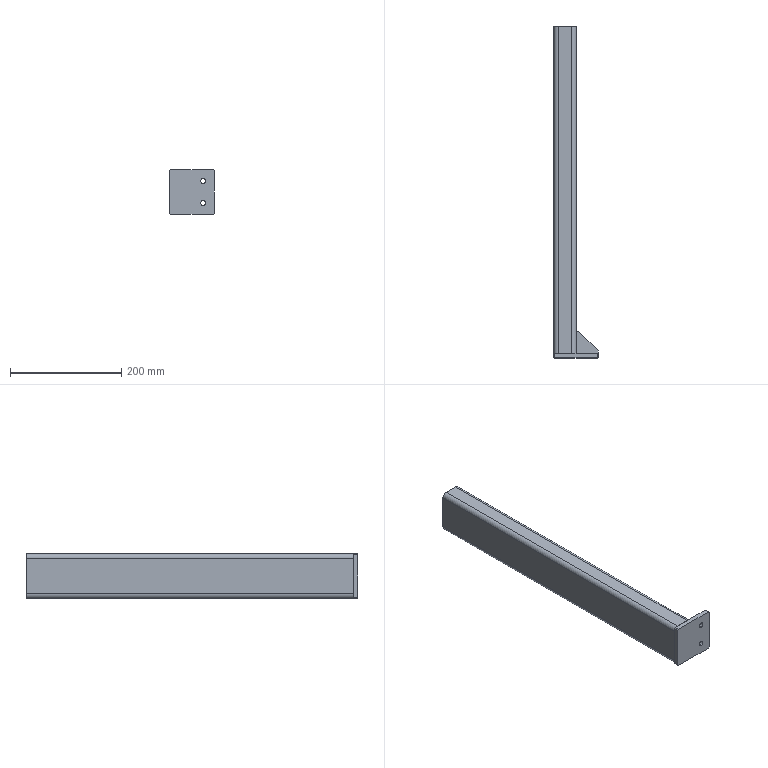Part | SolidWorks | features BaseBody 4 | 4 solids | 57 faces | box 80 x 598 x 80 mm | volume 570419 mm3 | plane 33 | cylinder 24 | commonest cylinder face diameters 5 x4 6 x4 6.8 x4 8 x4 9 x4 16 x4